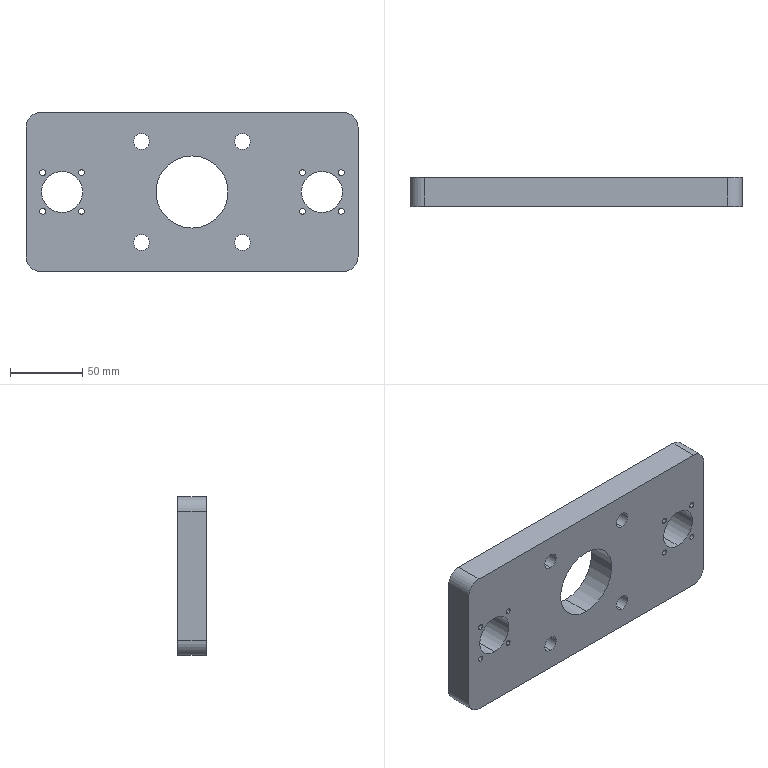Part | SolidWorks | features ICE 3, HoleWzd 2, LPattern 2, Extrusion 1, Fillet 1 | 1 solid | 52 faces | box 230 x 20 x 110 mm | volume 424729 mm3 | cylinder 40 | cone 6 | plane 6 | commonest cylinder face diameters 4 x16 11 x8 10.2 x6 20 x4 28.5 x4 50 x2